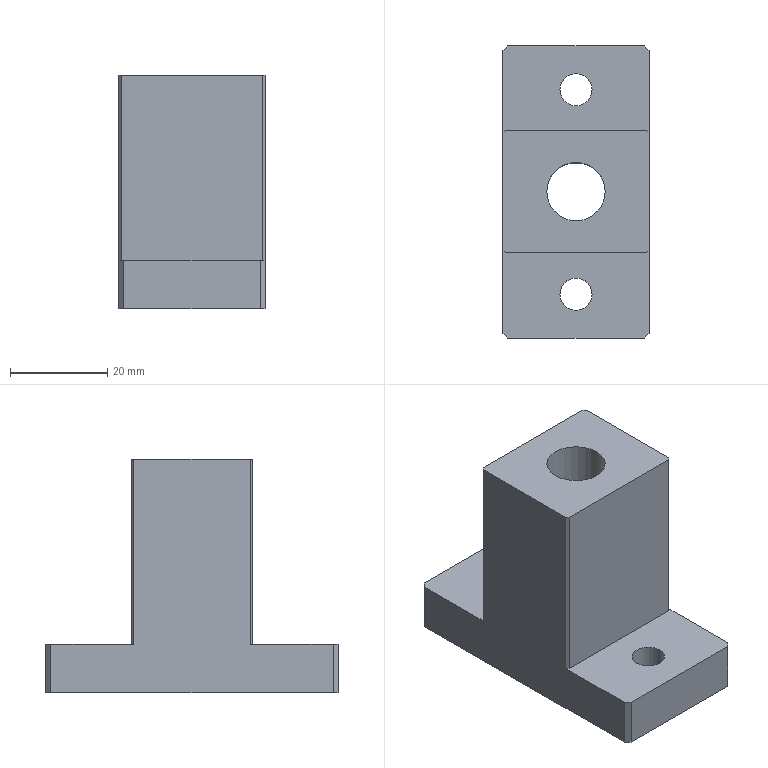NC program | NX | posted with a generic post | part box 30 x 60 x 48 mm
Lines 19 to 828 of 6343:
(ADAPTIVE_MILLING , TOOL : D16开粗)
N36 T02 M6
N38 G53
N40 G17 G0 G90 X13.985 Y-33.061 S4500 M3
N42 G43 Z20. H2
N44 Z-21.5
N46 G94 G1 X13.997 Y-32.911 Z-22.437 F2000.
N48 X14.008 Y-32.762 Z-22.808
N50 X14.02 Y-32.612 Z-23.08
N52 X14.032 Y-32.463 Z-23.3
N54 X14.043 Y-32.313 Z-23.484
N56 X14.055 Y-32.163 Z-23.642
N58 X14.066 Y-32.014 Z-23.78
N60 X14.078 Y-31.864 Z-23.9
N62 X14.09 Y-31.715 Z-24.005
N64 X14.101 Y-31.565 Z-24.098
N66 X14.113 Y-31.416 Z-24.179
N68 X14.124 Y-31.266 Z-24.25
N70 X14.136 Y-31.117 Z-24.31
N72 X14.148 Y-30.967 Z-24.362
N74 X14.159 Y-30.818 Z-24.405
N76 X14.171 Y-30.668 Z-24.439
N78 X14.182 Y-30.518 Z-24.466
N80 X14.194 Y-30.369 Z-24.485
N82 X14.206 Y-30.219 Z-24.496
N84 X14.217 Y-30.07 Z-24.5
N86 X14.398 Y-27.739
N88 G3 X13.137 Y-26.036 R1.616
N90 X9.412 Y-25.777 R24.281
N92 X-0.734 Y-25.732 R697.896
N94 G1 X-30.958 Y-25.731
N96 G2 X-37.538 Y-22.475 R8.77
N98 X-40.134 Y-16.806 R12.653
N100 X-40.681 Y-10.764 R34.184
N102 X-40.732 Y-1.127 R669.039
N104 G1 Y15.957
N106 G2 X-37.534 Y22.489 R8.758
N108 X-31.846 Y25.126 R12.591
N110 X-25.692 Y25.682 R34.318
N112 X-15.792 Y25.731 R681.956
N114 G1 X31.008 Y25.73
N116 G2 X37.564 Y22.421 R8.799
N118 X40.159 Y16.623 R12.811
N120 X40.675 Y10.615 R35.642
N122 X40.726 Y1.053 R672.132
N124 G1 X40.73 Y-16.005
N126 G2 X37.463 Y-22.534 R8.798
N128 X31.635 Y-25.165 R12.766
N130 X25.59 Y-25.684 R35.599
N132 X14.528 Y-25.699 R311.814
N134 G3 X2.143 Y-25.436 R215.264
N136 G1 X-2.721 Y-25.432
N138 X-28.82 Y-25.431
N140 G2 X-37.62 Y-20.592 R10.542
N142 X-39.919 Y-14.371 R15.604
N144 X-40.396 Y-7.344 R49.216
N146 X-40.432 Y2.331 R704.073
N148 X-40.415 Y14.381 R900.164
N150 X-35.438 Y22.722 R10.577
N152 X-29.3 Y24.931 R15.789
N154 X-22.759 Y25.388 R47.527
N156 X-13.272 Y25.431 R682.01
N158 G1 X28.909 Y25.429
N160 G2 X37.649 Y20.527 R10.565
N162 X39.898 Y14.435 R15.616
N164 X40.384 Y7.596 R47.272
N166 X40.426 Y-0.879 R651.896
N168 G1 X40.429 Y-13.942
N170 G2 X35.505 Y-22.67 R10.573
N172 X29.272 Y-24.933 R15.754
N174 X22.468 Y-25.393 R49.067
N176 X10.571 Y-25.235 R193.645
N178 G3 X-4.221 Y-25.133 R631.9
N180 G1 X-26.833 Y-25.132
N182 G2 X-34.196 Y-22.891 R11.955
N184 X-38.714 Y-16.566 R13.143
N186 X-39.917 Y-10.133 R24.645
N188 X-40.127 Y-0.912 R142.954
N190 G1 X-40.131 Y3.213
N192 G2 X-40.105 Y12.881 R446.004
N194 X-34.03 Y22.594 R11.722
N196 X-27.673 Y24.645 R17.928
N198 X-20.08 Y25.099 R59.176
N200 G1 X-10.292 Y25.13
N202 X27.109 Y25.128
N204 G2 X37.607 Y18.984 R11.777
N206 X39.675 Y12.391 R18.262
N208 X40.094 Y4.945 R62.435
N210 G1 X40.127 Y-3.717
N212 G2 X40.109 Y-12.742 R557.067
N214 X33.941 Y-22.639 R11.75
N216 X27.461 Y-24.673 R18.207
N218 X20.091 Y-25.098 R60.787
N220 X10.667 Y-24.942 R212.309
N222 G3 X-8.526 Y-24.831 R891.393
N224 G1 X-25.076 Y-24.832
N226 G2 X-30.535 Y-24.019 R15.261
N228 X-37.592 Y-17.472 R12.793
N230 X-39.431 Y-10.701 R20.839
N232 X-39.803 Y-3.064 R74.418
N234 X-39.81 Y11.306 R828.307
N236 X-32.781 Y22.436 R12.646
N238 X-26.044 Y24.388 R20.09
N240 X-18.484 Y24.797 R67.906
N242 G1 X-8.209 Y24.83
N244 X25.383 Y24.829
N246 G2 X31.373 Y23.668 R14.163
N248 X37.734 Y17.148 R12.98
N250 X39.442 Y10.527 R21.446
N252 X39.807 Y1.989 R85.035
N254 X39.808 Y-11.28 R817.076
N256 X32.83 Y-22.406 R12.643
N258 X26.099 Y-24.379 R19.982
N260 X17.152 Y-24.782 R68.08
N262 G1 X8.555 Y-24.604
N264 G3 X-8.341 Y-24.531 R937.351
N266 G1 X-23.541 Y-24.532
N268 G2 X-28.672 Y-23.994 R19.157
N270 X-37.04 Y-17.071 R13.264
N272 X-39.047 Y-10.188 R20.967
N274 X-39.495 Y-2.18 R69.441
N276 X-39.504 Y10.119 R511.825
N278 X-37.248 Y17.517 R13.897
N280 X-30.415 Y22.78 R14.226
N282 X-23.613 Y24.222 R25.275
N284 X-15.07 Y24.513 R106.766
N286 G1 X-6.37 Y24.53
N288 X23.396
N290 G2 X28.531 Y24.026 R19.801
N292 X36.977 Y17.17 R13.244
N294 X39.033 Y10.225 R20.826
N296 X39.49 Y2.105 R69.522
N298 X39.502 Y-10.082 R531.534
N300 X37.302 Y-17.429 R13.951
N302 X30.444 Y-22.765 R14.195
N304 X23.608 Y-24.221 R25.24
N306 X14.54 Y-24.423 R84.71
N308 G3 X-8.531 Y-24.231 R922.481
N310 G1 X-22.518 Y-24.23
N312 G2 X-27.981 Y-23.628 R20.413
N314 X-36.631 Y-16.463 R13.799
N316 X-38.719 Y-9.334 R21.731
N318 X-39.194 Y-0.915 R71.944
N320 X-39.186 Y9.284 R263.237
N322 X-37.093 Y16.518 R14.808
N324 X-30.049 Y22.28 R14.555
N326 X-22.94 Y23.88 R25.371
N328 X-14.249 Y24.208 R101.589
N330 G1 X-5.399 Y24.229
N332 X21.933 Y24.23
N334 G2 X27.047 Y23.848 R24.743
N336 X36.656 Y16.392 R13.805
N338 X38.721 Y9.251 R21.919
N340 X39.186 Y1.018 R72.061
N342 X39.184 Y-9.256 R266.644
N344 X37.121 Y-16.464 R14.839
N346 X30.089 Y-22.26 R14.533
N348 X22.907 Y-23.88 R25.251
N350 X14.139 Y-24.102 R81.497
N352 G3 X-8.346 Y-23.932 R949.844
N354 G1 X-20.945 Y-23.931
N356 G2 X-26.246 Y-23.53 R26.529
N358 X-36.275 Y-15.805 R14.288
N360 X-38.4 Y-8.491 R22.6
N362 X-38.892 Y0.227 R74.792
N364 X-38.874 Y8.401 R170.675
N366 X-36.954 Y15.505 R15.768
N368 X-29.762 Y21.764 R14.828
N370 X-22.685 Y23.5 R24.859
N372 X-14.11 Y23.897 R87.742
N374 G1 X-3.31 Y23.929
N376 X20.696
N378 G2 X26. Y23.573 R28.458
N380 X36.295 Y15.743 R14.306
N382 X38.39 Y8.499 R22.653
N384 X38.883 Y0.006 R73.152
N386 X38.869 Y-8.431 R168.888
N388 X36.862 Y-15.658 R15.689
N390 X29.681 Y-21.795 R14.885
N392 X22.408 Y-23.522 R25.086
N394 X13.717 Y-23.782 R78.693
N396 G3 X-6.7 Y-23.633 R943.214
N398 G1 X-18.846 Y-23.632
N400 G2 X-24.275 Y-23.41 R42.271
N402 X-36.061 Y-14.904 R14.836
N404 X-38.111 Y-7.488 R23.928
N406 X-38.587 Y1.082 R77.905
N408 X-38.534 Y7.98 R95.215
N410 X-36.233 Y15.514 R15.953
N412 X-28.816 Y21.544 R15.463
N414 X-21.38 Y23.237 R26.848
N416 X-12.203 Y23.603 R104.342
N418 G1 X-1.928 Y23.628
N420 X19.27 Y23.629
N422 G2 X24.806 Y23.328 R34.894
N424 X35.949 Y15.109 R14.776
N426 X38.052 Y7.863 R23.264
N428 X38.575 Y-0.628 R71.689
N430 X38.548 Y-7.714 R111.761
N432 X36.58 Y-14.922 R16.381
N434 X29.186 Y-21.385 R15.239
N436 X21.705 Y-23.187 R25.366
N438 X12.751 Y-23.458 R82.696
N440 G3 X-7. Y-23.334 R988.506
N442 G2 X-20.721 Y-23.302 R899.033
N444 X-27.094 Y-22.252 R20.326
N446 X-35.58 Y-14.577 R15.164
N448 X-37.729 Y-7.226 R23.748
N450 X-38.275 Y1.414 R71.809
N452 X-38.183 Y7.635 R63.011
N454 X-35.512 Y15.502 R16.099
N456 X-27.958 Y21.296 R16.05
N458 X-20.472 Y22.937 R28.199
N460 X-11.257 Y23.301 R108.51
N462 G1 X-0.607 Y23.328
N464 X17.958
N466 G2 X23.61 Y23.079 R42.712
N468 X35.635 Y14.444 R15.236
N470 X37.746 Y7.041 R24.133
N472 X38.277 Y-1.825 R75.703
N474 X38.139 Y-8.045 R53.534
N476 X34.713 Y-16.552 R15.623
N478 X27.152 Y-21.585 R16.639
N480 X19.537 Y-22.981 R30.011
N482 X12.715 Y-23.144 R99.556
N484 G1 X11.999 Y-23.2
N486 X-12.585 Y-23.177
N488 G3 X-19.482 Y-23.014 R161.863
N490 G2 X-25.671 Y-22.184 R23.424
N492 X-35.242 Y-13.99 R15.516
N494 X-37.422 Y-6.451 R24.486
N496 X-37.976 Y2.751 R75.299
N498 X-37.619 Y8.769 R32.43
N500 X-28.97 Y20.251 R15.524
N502 X-21.322 Y22.438 R24.622
N504 X-14.031 Y22.95 R73.993
N506 X-12. Y23.2 R11.124
N508 G1 X12.001
N510 G3 X18.628 Y23.027 R100.993
N512 G2 X24.553 Y22.469 R28.394
N514 X35.243 Y13.967 R15.529
N516 X37.411 Y6.468 R24.516
N518 X37.973 Y-2.921 R75.804
N520 X37.577 Y-8.973 R30.955
N522 X28.874 Y-20.292 R15.521
N524 X21.133 Y-22.432 R24.39
N526 X14.448 Y-22.826 R68.42
N528 G1 X13.282 Y-23.099
N530 X12.683 Y-23.146
N532 G3 X11.456 Y-23.888 R1.601
N534 G1 X11.051 Y-24.53
N536 X9.594 Y-26.84 Z-24.414
N538 X9.457 Y-27.023 Z-24.407
N540 X9.298 Y-27.187 Z-24.4
N542 G2 X8.243 Y-27.586 R1.603 F15000.
N544 G1 X-8.145 Y-27.617
N546 G2 X-9.243 Y-27.183 R1.602
N548 X-9.582 Y-26.743 Z-24.417 R2.039 F2000.
N550 G1 X-10.991 Y-24.52 Z-24.5
N552 X-11.231 Y-24.139
N554 X-11.483 Y-23.765
N556 G3 X-12.585 Y-23.177 R1.602
N558 G2 X-14.336 Y-22.942 R125.352
N560 G3 X-19.799 Y-22.688 R153.105
N562 G2 X-26.362 Y-21.418 R20.991
N564 X-34.947 Y-13.341 R15.923
N566 X-37.128 Y-5.612 R25.402
N568 X-37.571 Y5.765 R66.033
N570 X-35.46 Y13.367 R17.798
N572 X-27.641 Y20.268 R16.251
N574 X-19.997 Y22.205 R26.964
N576 X-15.115 Y22.606 R140.
N578 G1 X-13.859 Y22.985
N580 G3 X-12.785 Y24.897 R1.6
N582 X-13.653 Y25.958 Z-24.456 R1.612
N584 G1 X-15.255 Y26.718 Z-24.4
N586 X-17.86 Y27.953 F15000.
N588 G3 X-18.934 Y28.06 R1.603
N590 G1 X-21.765 Y27.356
N592 X-24.592 Y26.634
N594 G3 X-31.413 Y23.938 R33.71
N596 X-34.577 Y21.978 R29.741
N598 G1 X-35.786 Y21.107
N600 G3 X-38.5 Y18.162 R12.09
N602 X-40.073 Y15.155 R16.174
N604 G1 X-40.854 Y13.19
N606 X-41.619 Y11.219
N608 G3 X-42.854 Y4.139 R20.917
N610 X-42.262 Y-3.79 R53.425
N612 G1 X-41.374 Y-9.704
N614 G3 X-38.481 Y-17.024 R17.512
N616 G1 X-37.47 Y-18.499
N618 X-36.446 Y-19.965
N620 G3 X-32.674 Y-23.7 R17.348
N622 G1 X-32.041 Y-24.157
N624 X-31.402 Y-24.606
N626 G3 X-28.369 Y-26.106 R13.531
N628 X-24.521 Y-27.097 R24.4
N630 G1 X-18.534 Y-28.126
N632 G3 X-17.637 Y-28.021 R1.608
N634 G1 X-14.891 Y-26.852
N636 X-13.039 Y-26.057 Z-24.463 F2000.
N638 G3 X-12.26 Y-25.216 Z-24.5 R1.6
N640 X-13.46 Y-23.051 R1.6
N642 X-17.33 Y-22.546 R23.076
N644 G2 X-22.824 Y-21.957 R39.87
N646 X-34.637 Y-12.742 R16.312
N648 X-36.786 Y-5.158 R25.805
N650 X-37.219 Y5.354 R54.785
N652 X-34.869 Y13.263 R17.807
N654 X-27.094 Y19.93 R16.614
N656 X-19.303 Y21.895 R27.6
N658 G3 X-15.78 Y22.292 R69.058
N660 X-14.94 Y22.646 R13.261
N662 X-13.858 Y24.522 R1.6
N664 X-14.708 Y25.606 Z-24.455 R1.612
N666 G1 X-16.289 Y26.391 Z-24.4
N668 X-18.797 Y27.636 F15000.
N670 G3 X-20.014 Y27.721 R1.602
N672 G1 X-26.407 Y25.59
N674 G3 X-32.132 Y22.742 R22.941
N676 G1 X-33.69 Y21.66
N678 G3 X-36.977 Y18.677 R20.671
N680 X-40.341 Y12.811 R17.594
N682 X-41.301 Y9.736 R39.249
N684 X-42.167 Y0.137 R30.252
N686 G1 X-41.751 Y-5.83
N688 G3 X-40.263 Y-12.321 R21.487
N690 X-37.873 Y-16.939 R25.734
N692 G1 X-36.842 Y-18.523
N694 X-35.799 Y-20.098
N696 G3 X-33.549 Y-22.314 R8.889
N698 G1 X-33.214 Y-22.527
N700 X-31.625 Y-23.484
N702 X-30.03 Y-24.429
N704 G3 X-23.352 Y-27.028 R25.37
N706 G1 X-19.065 Y-28.029
N708 G3 X-18.018 Y-27.918 R1.604
N710 G1 X-15.433 Y-26.698
N712 X-13.721 Y-25.884 Z-24.459 F2000.
N714 G3 X-12.936 Y-24.902 Z-24.5 R1.6
N716 X-13.991 Y-22.955 R1.6
N718 X-17.075 Y-22.351 R13.124
N720 G2 X-22.423 Y-21.631 R47.762
N722 X-34.388 Y-12.032 R16.731
N724 X-36.526 Y-4.133 R27.049
N726 X-36.839 Y5.183 R45.298
N728 X-34.06 Y13.486 R17.543
N730 X-26.132 Y19.774 R17.15
N732 X-18.72 Y21.582 R29.31
N734 G3 X-16.325 Y21.988 R15.841
N736 G1 X-16.188 Y22.048
N738 G3 X-15.527 Y23.613 R1.6
N740 X-16.249 Y24.709 Z-24.458 R1.616
N742 G1 X-17.799 Y25.694 Z-24.4
N744 X-19.825 Y26.981 F15000.
N746 G3 X-21.262 Y27.123 R1.601
N748 G1 X-23.209 Y26.369
N750 X-25.151 Y25.602
N752 G3 X-30.97 Y22.862 R67.452
N754 X-34.596 Y20.308 R19.289
N756 X-36.526 Y18.237 R16.679
N758 G1 X-37.319 Y17.228
N760 X-38.1 Y16.21
N762 G3 X-39.724 Y13.258 R13.969
N764 X-41.019 Y9.513 R40.696
N766 G1 X-41.251 Y8.713
N768 X-41.473 Y7.911
N770 G3 X-42.012 Y2.689 R18.213
N772 G1 X-41.93 Y0.698
N774 X-41.834 Y-1.291
N776 G3 X-40.686 Y-8.948 R45.233
N778 X-38.126 Y-15.582 R28.533
N780 G1 X-37.541 Y-16.68
N782 X-36.94 Y-17.769
N784 G3 X-34.37 Y-20.845 R12.645
N786 X-31.624 Y-22.846 R17.999
N788 X-28.803 Y-24.42 R39.769
N790 X-25.369 Y-25.858 R29.788
N792 G1 X-19.601 Y-27.857
N794 G3 X-18.359 Y-27.775 R1.602
N796 G1 X-15.907 Y-26.544
N798 X-14.222 Y-25.693 Z-24.459 F2000.
N800 G3 X-13.46 Y-24.683 Z-24.5 R1.6
N802 X-14.527 Y-22.783 R1.6
N804 X-18.114 Y-22.009 R17.004
N806 G2 X-23.865 Y-20.8 R30.869
N808 X-34.026 Y-11.582 R17.055
N810 X-36.214 Y-3.505 R27.507
N812 X-36.43 Y5.173 R37.702
N814 X-32.773 Y14.27 R17.148
N816 X-24.772 Y19.761 R18.042
N818 X-18.672 Y21.232 R34.723
N820 G3 X-16.646 Y21.741 R8.5
N822 G2 X-15.502 Y22.389 R6.054
N824 G3 X-14.922 Y24.776 R1.6
N826 X-16.007 Y25.412 Z-24.46 R1.617
N828 G1 X-17.889 Y25.65 Z-24.4
N830 X-21.009 Y26.046 F15000.
N832 G3 X-21.717 Y25.977 R1.62
N834 G1 X-23.54 Y25.372
N836 X-25.358 Y24.752
N838 G3 X-30.021 Y22.666 R34.525
N840 X-32.045 Y21.528 R36.787
N842 X-34.586 Y19.68 R21.25
N844 X-36.876 Y17.097 R13.217
N846 X-38.139 Y15.155 R36.145
N848 X-40.633 Y8.803 R22.047
N850 X-41.158 Y5.127 R23.446
N852 G1 X-41.278 Y3.24
N854 X-41.382 Y1.352
N856 G3 X-41.212 Y-2.802 R29.864
N858 X-40.793 Y-5.746 R43.313
N860 G1 X-40.556 Y-7.085
N862 X-40.303 Y-8.421
N864 G3 X-37.705 Y-15.071 R22.03
N866 G1 X-37.046 Y-16.188
N868 X-36.373 Y-17.296
N870 G3 X-28.217 Y-24.209 R18.238
N872 G1 X-20.079 Y-27.704
N874 G3 X-18.651 Y-27.622 R1.601
N876 G1 X-16.456 Y-26.363
N878 X-14.817 Y-25.418 Z-24.459 F2000.
N880 G3 X-14.113 Y-24.372 Z-24.5 R1.6
N882 X-15.004 Y-22.63 R1.6
N884 X-17.509 Y-21.901 R10.047
N886 G2 X-22.695 Y-20.742 R47.018
N888 X-33.836 Y-10.771 R17.575
N890 X-35.954 Y-2.437 R28.718
N892 X-35.947 Y5.566 R30.814
N894 X-26.592 Y18.431 R16.818
N896 X-20.24 Y20.552 R26.748
N898 G3 X-17.265 Y21.323 R21.278
N900 X-16.515 Y21.819 R13.252
N902 X-16.049 Y23.932 R1.6
N904 X-17.183 Y24.71 Z-24.455 R1.612
N906 G1 X-18.929 Y24.987 Z-24.4
N908 X-21.973 Y25.47 F15000.
N910 G3 X-22.73 Y25.407 R1.615
N912 G1 X-23.99 Y24.989
N914 X-25.246 Y24.558
N916 G3 X-28.257 Y23.183 R21.907
N918 G1 X-29.827 Y22.321
N920 X-31.388 Y21.444
N922 G3 X-35.425 Y18.012 R16.248
N924 G1 X-36.113 Y17.198
N926 X-36.774 Y16.363
N928 G3 X-39.33 Y11.532 R18.791
N930 G1 X-39.541 Y10.905
N932 X-39.734 Y10.272
N934 X-40.097 Y8.998
N936 X-40.449 Y7.722
N938 G3 X-41.155 Y2.48 R22.513
N940 X-41.076 Y0.496 R21.014
N942 G1 X-40.867 Y-1.885
N944 X-40.64 Y-4.263
N946 G3 X-38.015 Y-13.354 R28.652
N948 X-35.093 Y-18.048 R26.436
N950 X-33.504 Y-19.942 R22.055
N952 X-29.463 Y-23.094 R18.103
N954 X-24.248 Y-25.326 R21.203
N956 G1 X-21.49 Y-26.09
N958 G3 X-20.877 Y-26.137 R1.636
N960 G1 X-17.725 Y-25.768
N962 X-15.685 Y-25.524 Z-24.464 F2000.
N964 G3 X-14.723 Y-24.968 Z-24.5 R1.6
N966 X-15.276 Y-22.502 R1.6
N968 X-18.076 Y-21.581 R12.064
N970 G2 X-23.311 Y-20.103 R38.542
N972 X-33.51 Y-10.276 R18.002
N974 X-35.667 Y-1.458 R28.912
N976 X-35.335 Y6.379 R25.562
N978 X-26.411 Y17.937 R16.882
N980 X-20.538 Y20.089 R27.825
N982 G3 X-17.668 Y20.981 R19.027
N984 G1 X-17.358 Y21.19
N986 G3 X-17.035 Y23.074 R1.6
N988 X-18.107 Y23.909 Z-24.456 R1.612
N990 G1 X-19.849 Y24.305 Z-24.4
N992 X-22.503 Y24.908 F15000.
N994 G3 X-23.573 Y24.779 R1.603
N996 G1 X-28.872 Y22.129
N998 G3 X-33.661 Y18.678 R18.432
N1000 X-35.27 Y17.005 R33.055
N1002 X-37.9 Y13.197 R21.61
N1004 X-39.891 Y8.298 R22.121
N1006 G1 X-40.166 Y7.172
N1008 X-40.419 Y6.04
N1010 G3 X-40.733 Y0.792 R19.406
N1012 G1 X-40.556 Y-1.567
N1014 X-40.363 Y-3.925
N1016 G3 X-38.933 Y-10.284 R27.332
N1018 X-36.914 Y-14.434 R22.314
N1020 X-35.593 Y-16.479 R38.426
N1022 X-31.23 Y-21.232 R25.098
N1024 G1 X-30.418 Y-21.916
N1026 X-29.598 Y-22.591
N1028 G3 X-24.843 Y-25.024 R14.267
N1030 G1 X-21.965 Y-25.866
N1032 G3 X-21.327 Y-25.92 R1.631
N1034 G1 X-18.135 Y-25.54
N1036 X-16.153 Y-25.299 Z-24.463 F2000.
N1038 G3 X-15.158 Y-24.694 Z-24.5 R1.6
N1040 X-15.751 Y-22.278 R1.6
N1042 X-18.547 Y-21.25 R13.8
N1044 G2 X-24.062 Y-19.329 R34.092
N1046 X-33.304 Y-9.517 R18.534
N1048 X-35.243 Y4.194 R28.456
N1050 X-26.061 Y17.536 R17.07
N1052 X-20.945 Y19.578 R29.38
N1054 G3 X-18.012 Y20.638 R19.272
N1056 X-17.205 Y21.337 R4.301
N1058 G1 X-17.051 Y21.444
N1060 G3 X-16.545 Y23.484 R1.6
N1062 X-17.643 Y24.321 Z-24.455 R1.612
N1064 G1 X-19.367 Y24.68 Z-24.4
N1066 X-22.086 Y25.245 F15000.
N1068 G3 X-23.266 Y25.032 R1.602
N1070 G1 X-30.01 Y20.779
N1072 G3 X-34.014 Y17.617 R23.509
N1074 X-35.838 Y15.451 R17.459
N1076 X-37.145 Y13.539 R33.942
N1078 X-39.098 Y9.367 R20.159
N1080 X-39.79 Y7.165 R33.389
N1082 X-40.382 Y0.666 R19.748
N1084 G1 X-40.244 Y-1.197
N1086 X-40.091 Y-3.058
N1088 G3 X-38.708 Y-9.431 R28.559
N1090 X-36.749 Y-13.611 R22.829
N1092 G1 X-36.069 Y-14.75
N1094 X-35.376 Y-15.882
N1096 G3 X-29.928 Y-21.564 R20.875
N1098 X-27.106 Y-23.271 R21.988
N1100 G1 X-22.182 Y-25.765
N1102 G3 X-21.182 Y-25.913 R1.604
N1104 G1 X-18.336 Y-25.413
N1106 X-16.469 Y-25.08 Z-24.459 F2000.
N1108 G3 X-15.454 Y-24.339 Z-24.5 R1.6
N1110 X-15.967 Y-22.176 R1.6
N1112 X-18.238 Y-21.145 R9.49
N1114 G2 X-23.225 Y-19.276 R48.494
N1116 X-33.127 Y-8.686 R19.155
N1118 X-34.817 Y3.943 R26.45
N1120 X-26.011 Y16.978 R17.126
N1122 X-20.505 Y19.348 R34.658
N1124 G3 X-18.285 Y20.324 R11.429
N1126 G1 X-17.735 Y20.833
N1128 G3 X-17.393 Y22.683 R1.6
N1130 X-18.421 Y23.538 Z-24.457 R1.612
N1132 G1 X-20.168 Y24.008 Z-24.4
N1134 X-22.605 Y24.664 F15000.
N1136 G3 X-23.95 Y24.421 R1.601
N1138 G1 X-30.434 Y19.794
N1140 G3 X-33.623 Y17.403 R87.827
N1142 X-36.229 Y14.469 R11.135
N1144 X-37.397 Y12.472 R32.023
N1146 X-39.103 Y7.778 R19.601
N1148 X-39.897 Y1.102 R28.488
N1150 G1 Y-0.069
N1152 X-39.885 Y-1.239
N1154 G3 X-38.724 Y-7.808 R23.78
N1156 X-36.991 Y-11.917 R25.967
N1158 G1 X-36.171 Y-13.478
N1160 X-35.336 Y-15.031
N1162 G3 X-30.682 Y-20.547 R20.237
N1164 X-27.424 Y-22.792 R21.813
N1166 G1 X-22.497 Y-25.562
N1168 G3 X-21.422 Y-25.741 R1.603
N1170 G1 X-18.631 Y-25.224
N1172 X-16.771 Y-24.874 Z-24.459 F2000.
N1174 G3 X-15.76 Y-24.121 Z-24.5 R1.6
N1176 X-16.283 Y-21.974 R1.6
N1178 X-18.928 Y-20.688 R12.622
N1180 G2 X-24.187 Y-18.325 R37.275
N1182 X-32.972 Y-7.779 R19.767
N1184 X-34.366 Y3.801 R24.59
N1186 X-26.001 Y16.392 R17.177
N1188 X-20.807 Y18.867 R36.139
N1190 G3 X-18.648 Y19.929 R11.394
N1192 G1 X-18.189 Y20.402
N1194 G3 X-18.243 Y22.771 R1.6
N1196 X-19.516 Y23.146 Z-24.457 R1.616
N1198 G1 X-21.318 Y22.89 Z-24.4
N1200 X-24.613 Y22.421 F15000.
N1202 G3 X-25.121 Y22.259 R1.685
N1204 G1 X-26.298 Y21.654
N1206 X-27.469 Y21.037
N1208 G3 X-30.227 Y19.228 R22.295
N1210 G1 X-31.807 Y18.019
N1212 X-33.376 Y16.795
N1214 X-33.888 Y16.374
N1216 X-34.389 Y15.94
N1218 G3 X-35.384 Y14.642 R5.403
N1220 X-37.614 Y10.208 R51.315
N1222 X-38.739 Y6.416 R15.949
N1224 G1 X-39.039 Y4.621
N1226 X-39.323 Y2.824
N1228 G3 X-39.167 Y-3.917 R22.101
N1230 X-38.014 Y-8.223 R24.955
N1232 G1 X-37.559 Y-9.47
N1234 X-37.089 Y-10.712
N1236 G3 X-34.28 Y-15.527 R19.852
N1238 X-30.883 Y-19.615 R71.007
N1240 X-26.824 Y-22.959 R17.527
N1242 G1 X-22.94 Y-25.279
N1244 G3 X-21.817 Y-25.477 R1.603
N1246 G1 X-19.059 Y-24.947
N1248 X-17.205 Y-24.586 Z-24.459 F2000.
N1250 G3 X-16.198 Y-23.822 Z-24.5 R1.6
N1252 X-16.725 Y-21.691 R1.6
N1254 X-19.124 Y-20.39 R12.528
N1256 G2 X-24.241 Y-17.82 R39.626
N1258 X-32.828 Y-6.802 R20.394
N1260 X-33.867 Y3.884 R22.783
N1262 X-26.139 Y15.704 R17.199
N1264 X-21.117 Y18.36 R36.292
N1266 G3 X-18.971 Y19.535 R11.219
N1268 G1 X-18.476 Y20.091
N1270 G3 X-18.564 Y22.274 R1.6
N1272 X-19.859 Y22.726 Z-24.456 R1.612
N1274 G1 X-21.621 Y22.538 Z-24.4
N1276 X-24.691 Y22.208 F15000.
N1278 G3 X-25.408 Y21.949 R1.615
N1280 G1 X-29.555 Y19.184
N1282 G3 X-33.922 Y15.2 R19.584
N1284 X-35.344 Y13.367 R32.297
N1286 X-37.604 Y9.018 R18.383
N1288 X-38.09 Y7.389 R18.072
N1290 G1 X-38.407 Y6.102
N1292 X-38.71 Y4.812
N1294 G3 X-38.965 Y-2.369 R20.893
N1296 X-36.892 Y-10.001 R30.973
N1298 X-34.801 Y-14.122 R24.325
N1300 X-32.695 Y-16.913 R23.511
N1302 X-28.47 Y-20.942 R31.009
N1304 G1 X-23.166 Y-25.12
N1306 G3 X-21.78 Y-25.414 R1.601
N1308 G1 X-19.296 Y-24.78
N1310 X-17.469 Y-24.308 Z-24.459 F2000.
N1312 G3 X-16.509 Y-23.484 Z-24.5 R1.6
N1314 X-16.951 Y-21.532 R1.6
N1316 X-19.509 Y-19.983 R12.528
N1318 G2 X-24.662 Y-17.053 R37.923
N1320 X-32.899 Y-4.975 R21.081
N1322 X-33.139 Y4.972 R20.52
N1324 X-26.183 Y15.059 R17.279
N1326 X-21.407 Y17.838 R36.801
N1328 G3 X-19.35 Y19.069 R11.958
N1330 G1 X-19.174 Y19.264
N1332 G3 X-19.313 Y21.319 R1.6
N1334 X-20.606 Y21.803 Z-24.455 R1.612
N1336 G1 X-22.361 Y21.648 Z-24.4
N1338 X-25.359 Y21.384 F15000.
N1340 G3 X-26.106 Y21.121 R1.614
N1342 G1 X-29.428 Y18.906
N1344 G3 X-34.676 Y13.22 R16.448
N1346 X-37.802 Y6.999 R65.625
N1348 X-38.808 Y1.272 R12.467
N1350 G1 X-38.725 Y-0.094
N1352 X-38.629 Y-1.46
N1354 G3 X-36.648 Y-9.367 R25.96
N1356 X-35.306 Y-12.021 R24.729
N1358 G1 X-32.135 Y-17.447
N1360 G3 X-27.348 Y-21.722 R10.429
N1362 G1 X-24.264 Y-23.086
N1364 X-24.072 Y-23.155
N1366 X-23.873 Y-23.202
N1368 X-20.478 Y-23.753
N1370 X-18.495 Y-24.069 Z-24.463 F2000.
N1372 G3 X-17.381 Y-23.77 Z-24.5 R1.6
N1374 X-17.332 Y-21.229 R1.6
N1376 X-19.49 Y-19.768 R11.108
N1378 G2 X-24.368 Y-16.774 R45.598
N1380 X-33.073 Y2.293 R21.394
N1382 X-26.521 Y14.167 R17.176
N1384 X-21.642 Y17.323 R35.757
N1386 G3 X-19.534 Y18.737 R11.279
N1388 X-19.114 Y19.351 R6.05
N1390 G1 X-18.845 Y19.663
N1392 G3 X-18.955 Y21.867 R1.6
N1394 X-20.254 Y22.295 Z-24.456 R1.612
N1396 G1 X-22.017 Y22.078 Z-24.4
N1398 X-25.257 Y21.677 F15000.
N1400 G3 X-25.777 Y21.52 R1.679
N1402 G1 X-26.37 Y21.225
N1404 X-26.958 Y20.919
N1406 G3 X-28.234 Y19.895 R5.451
N1408 G1 X-29.839 Y18.154
N1410 X-31.433 Y16.402
N1412 G3 X-34.488 Y12.199 R29.128
N1414 X-37.299 Y6.937 R62.025
N1416 X-38.408 Y1.25 R11.709
N1418 G1 X-38.33 Y-0.116
N1420 X-38.239 Y-1.482
N1422 G3 X-34.897 Y-12.035 R25.237
N1424 G1 X-34.039 Y-13.503
N1426 X-33.169 Y-14.963
N1428 G3 X-27.92 Y-20.476 R19.355
N1430 G1 X-24.47 Y-22.897
N1432 G3 X-23.754 Y-23.175 R1.614
N1434 G1 X-20.67 Y-23.569
N1436 X-19.701 Y-23.695 Z-24.431 F2000.
N1438 X-18.731 Y-23.811 Z-24.461
N1440 G3 X-17.587 Y-23.436 Z-24.5 R1.599
N1442 X-17.539 Y-21.04 R1.6
N1444 X-19.852 Y-19.325 R12.495
N1446 G2 X-24.831 Y-15.912 R42.957
N1448 X-32.666 Y0.691 R21.185
N1450 X-26.636 Y13.405 R17.145
N1452 X-21.884 Y16.781 R35.487
N1454 G3 X-19.786 Y18.311 R12.428
N1456 G1 X-19.353 Y18.968
N1458 G3 X-19.513 Y20.875 R1.6
N1460 X-20.754 Y21.413 Z-24.456 R1.612
N1462 G1 X-22.547 Y21.365 Z-24.4
N1464 X-25.196 Y21.293 F15000.
N1466 G3 X-26.284 Y20.825 R1.602
N1468 G1 X-31.218 Y15.892
N1470 G3 X-34.777 Y11.16 R21.151
N1472 X-35.771 Y9.277 R29.682
N1474 X-37.028 Y5.324 R17.287
N1476 X-37.368 Y2.699 R20.622
N1478 X-37.478 Y0.218 R36.859
N1480 X-37.051 Y-4.215 R23.33
N1482 G1 X-36.801 Y-5.518
N1484 X-36.535 Y-6.817
N1486 G3 X-33.635 Y-13.42 R19.671
N1488 X-31.123 Y-16.474 R21.157
N1490 G1 X-29.595 Y-18.012
N1492 X-28.06 Y-19.543
N1494 G3 X-24.791 Y-22.594 R130.042
N1496 X-23.868 Y-23.007 R1.604
N1498 G1 X-20.953 Y-23.296
N1500 X-19.994 Y-23.395 Z-24.43 F2000.
N1502 X-19.034 Y-23.481 Z-24.46
N1504 G3 X-17.882 Y-23.055 Z-24.5 R1.599
N1506 X-17.859 Y-20.737 R1.6
N1508 X-20.094 Y-18.928 R13.285
N1510 G2 X-24.936 Y-15.302 R45.046
N1512 X-32.037 Y-2.004 R21.332
N1514 X-26.764 Y12.591 R17.095
N1516 X-22.105 Y16.226 R34.927
N1518 G3 X-20.02 Y17.879 R12.791
N1520 G1 X-19.834 Y18.16
N1522 G3 X-20.066 Y19.934 R1.6
N1524 X-21.262 Y20.475 Z-24.458 R1.616
N1526 G1 X-23.099 Y20.48 Z-24.4
N1528 X-25.63 Y20.486 F15000.
N1530 G3 X-26.766 Y20.018 R1.602
N1532 G1 X-28.088 Y18.699
N1534 X-29.4 Y17.37
N1536 G3 X-32.641 Y13.293 R29.525
N1538 G1 X-33.605 Y11.839
N1540 X-34.555 Y10.375
N1542 G3 X-35.902 Y7.217 R12.326
N1544 X-36.934 Y2.355 R50.586
N1546 X-36.927 Y-3.535 R16.977
N1548 X-35.223 Y-9.225 R25.813
N1550 X-34.219 Y-11.439 R35.433
N1552 X-30.491 Y-16.678 R21.986
N1554 G1 X-25.183 Y-22.203
N1556 G3 X-24.158 Y-22.689 R1.603
N1558 G1 X-21.32 Y-22.919
N1560 X-19.432 Y-23.067 Z-24.459 F2000.
N1562 G3 X-18.261 Y-22.604 Z-24.5 R1.6
N1564 X-18.251 Y-20.346 R1.6
N1566 X-20.338 Y-18.508 R12.605
N1568 G2 X-24.926 Y-14.783 R47.652
N1570 X-31.262 Y-3.698 R21.506
N1572 X-26.769 Y11.858 R17.038
N1574 X-22.831 Y15.259 R31.359
N1576 G3 X-20.431 Y17.214 R23.777
N1578 X-19.776 Y18.288 R2.536
N1580 G1 X-19.657 Y18.479
N1582 G3 X-20.358 Y20.784 R1.6
N1584 X-21.667 Y20.786 Z-24.458 R1.616
N1586 G1 X-23.349 Y20.036 Z-24.4
N1588 X-26.833 Y18.479 F15000.
N1590 X-27.427 Y18.184
N1592 X-28.014 Y17.878
N1594 G3 X-29.291 Y16.854 R5.451
N1596 X-30.831 Y15.117 R35.076
N1598 X-32.361 Y12.957 R21.092
N1600 G1 X-33.322 Y11.405
N1602 X-34.268 Y9.845
N1604 G3 X-36.46 Y3.808 R18.788
N1606 X-36.53 Y-0.9 R15.586
N1608 G1 X-36.344 Y-2.256
N1610 X-36.146 Y-3.61
N1612 G3 X-32.773 Y-12.606 R24.896
N1614 X-31.251 Y-14.808 R35.648
N1616 X-28.291 Y-18.55 R70.567
N1618 G1 X-25.4 Y-21.957
N1620 G3 X-24.258 Y-22.52 R1.602
N1622 G1 X-21.553 Y-22.652
N1624 X-19.674 Y-22.739 Z-24.459 F2000.
N1626 G3 X-18.51 Y-22.228 Z-24.5 R1.6
N1628 X-18.469 Y-20.099 R1.6
N1630 X-20.801 Y-17.882 R14.908
N1632 G2 X-25.471 Y-13.67 R42.754
N1634 X-30.77 Y-3.617 R21.099
N1636 X-26.83 Y11.025 R16.907
N1638 X-22.378 Y15.162 R34.496
N1640 G3 X-20.317 Y17.105 R13.587
N1642 X-19.978 Y17.814 R5.404
N1644 X-20.649 Y19.826 R1.6
N1646 X-22.025 Y19.935 Z-24.455 R1.612
N1648 G1 X-23.67 Y19.302 Z-24.4